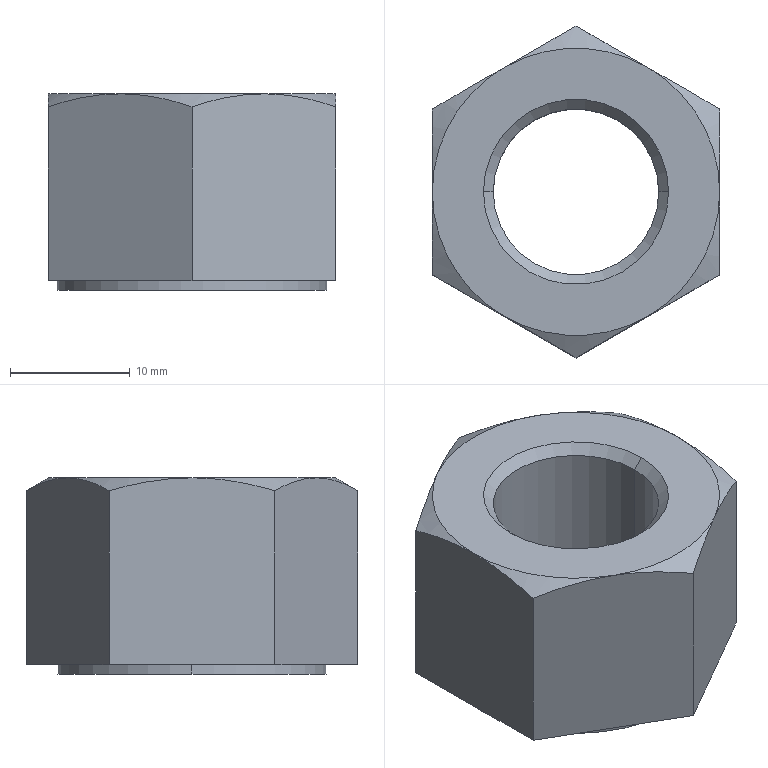Part | SolidWorks | features Cut 2, Chamfer 1, Extrusion 1 | 1 solid | 23 faces | box 24 x 27.713 x 16.4 mm | volume 5589 mm3 | cone 10 | plane 9 | cylinder 4 | commonest cylinder face diameters 13.835 x2 22.5 x2
STEP:
#1=CARTESIAN_POINT('',(-6.918,0.,15.58));
#2=VERTEX_POINT('',#1);
#3=CARTESIAN_POINT('',(6.918,0.,15.58));
#4=VERTEX_POINT('',#3);
#5=CARTESIAN_POINT('',(0.,0.,15.58));
#6=DIRECTION('',(0.,0.,1.));
#7=DIRECTION('',(-1.,0.,0.));
#8=AXIS2_PLACEMENT_3D('',#5,#6,#7);
#9=CIRCLE('',#8,6.918);
#10=EDGE_CURVE('',#2,#4,#9,.T.);
#11=ORIENTED_EDGE('',*,*,#10,.F.);
#12=CARTESIAN_POINT('',(-7.738,0.,16.4));
#13=VERTEX_POINT('',#12);
#14=CARTESIAN_POINT('',(-6.918,0.,15.58));
#15=DIRECTION('',(-0.7071,0.,0.7071));
#16=VECTOR('',#15,1000.);
#17=LINE('',#14,#16);
#18=EDGE_CURVE('',#2,#13,#17,.T.);
#19=ORIENTED_EDGE('',*,*,#18,.T.);
#20=CARTESIAN_POINT('',(7.738,0.,16.4));
#21=VERTEX_POINT('',#20);
#22=CARTESIAN_POINT('',(0.,0.,16.4));
#23=DIRECTION('',(0.,0.,-1.));
#24=DIRECTION('',(-1.,0.,0.));
#25=AXIS2_PLACEMENT_3D('',#22,#23,#24);
#26=CIRCLE('',#25,7.738);
#27=EDGE_CURVE('',#21,#13,#26,.T.);
#28=ORIENTED_EDGE('',*,*,#27,.F.);
#29=CARTESIAN_POINT('',(6.918,0.,15.58));
#30=DIRECTION('',(0.7071,0.,0.7071));
#31=VECTOR('',#30,1000.);
#32=LINE('',#29,#31);
#33=EDGE_CURVE('',#4,#21,#32,.T.);
#34=ORIENTED_EDGE('',*,*,#33,.F.);
#35=EDGE_LOOP('',(#11,#19,#28,#34));
#36=FACE_OUTER_BOUND('',#35,.T.);
#37=CARTESIAN_POINT('',(0.,0.,15.58));
#38=DIRECTION('',(0.,0.,1.));
#39=DIRECTION('',(1.,0.,0.));
#40=AXIS2_PLACEMENT_3D('',#37,#38,#39);
#41=CONICAL_SURFACE('',#40,6.918,0.7854);
#42=ADVANCED_FACE('',(#36),#41,.F.);
#43=CARTESIAN_POINT('',(6.918,0.,0.82));
#44=VERTEX_POINT('',#43);
#45=CARTESIAN_POINT('',(-6.918,0.,0.82));
#46=VERTEX_POINT('',#45);
#47=CARTESIAN_POINT('',(0.,0.,0.82));
#48=DIRECTION('',(0.,0.,-1.));
#49=DIRECTION('',(-1.,0.,0.));
#50=AXIS2_PLACEMENT_3D('',#47,#48,#49);
#51=CIRCLE('',#50,6.918);
#52=EDGE_CURVE('',#44,#46,#51,.T.);
#53=ORIENTED_EDGE('',*,*,#52,.F.);
#54=CARTESIAN_POINT('',(7.738,0.,0.));
#55=VERTEX_POINT('',#54);
#56=CARTESIAN_POINT('',(7.738,0.,0.));
#57=DIRECTION('',(0.7071,0.,-0.7071));
#58=VECTOR('',#57,1000.);
#59=LINE('',#56,#58);
#60=EDGE_CURVE('',#44,#55,#59,.T.);
#61=ORIENTED_EDGE('',*,*,#60,.T.);
#62=CARTESIAN_POINT('',(-7.738,0.,0.));
#63=VERTEX_POINT('',#62);
#64=CARTESIAN_POINT('',(0.,0.,0.));
#65=DIRECTION('',(0.,0.,1.));
#66=DIRECTION('',(-1.,0.,0.));
#67=AXIS2_PLACEMENT_3D('',#64,#65,#66);
#68=CIRCLE('',#67,7.738);
#69=EDGE_CURVE('',#63,#55,#68,.T.);
#70=ORIENTED_EDGE('',*,*,#69,.F.);
#71=CARTESIAN_POINT('',(-7.738,0.,0.));
#72=DIRECTION('',(-0.7071,0.,-0.7071));
#73=VECTOR('',#72,1000.);
#74=LINE('',#71,#73);
#75=EDGE_CURVE('',#46,#63,#74,.T.);
#76=ORIENTED_EDGE('',*,*,#75,.F.);
#77=EDGE_LOOP('',(#53,#61,#70,#76));
#78=FACE_OUTER_BOUND('',#77,.T.);
#79=CARTESIAN_POINT('',(0.,0.,0.));
#80=DIRECTION('',(0.,0.,-1.));
#81=DIRECTION('',(-1.,0.,0.));
#82=AXIS2_PLACEMENT_3D('',#79,#80,#81);
#83=CONICAL_SURFACE('',#82,7.738,0.7854);
#84=ADVANCED_FACE('',(#78),#83,.F.);
#85=CARTESIAN_POINT('',(11.25,0.,0.8));
#86=VERTEX_POINT('',#85);
#87=CARTESIAN_POINT('',(-11.25,0.,0.8));
#88=VERTEX_POINT('',#87);
#89=CARTESIAN_POINT('',(0.,0.,0.8));
#90=DIRECTION('',(0.,0.,1.));
#91=DIRECTION('',(1.,0.,0.));
#92=AXIS2_PLACEMENT_3D('',#89,#90,#91);
#93=CIRCLE('',#92,11.25);
#94=EDGE_CURVE('',#86,#88,#93,.T.);
#95=ORIENTED_EDGE('',*,*,#94,.F.);
#96=CARTESIAN_POINT('',(11.25,0.,0.));
#97=VERTEX_POINT('',#96);
#98=CARTESIAN_POINT('',(11.25,0.,0.8));
#99=DIRECTION('',(0.,0.,-1.));
#100=VECTOR('',#99,1000.);
#101=LINE('',#98,#100);
#102=EDGE_CURVE('',#86,#97,#101,.T.);
#103=ORIENTED_EDGE('',*,*,#102,.T.);
#104=CARTESIAN_POINT('',(-11.25,0.,0.));
#105=VERTEX_POINT('',#104);
#106=CARTESIAN_POINT('',(0.,0.,0.));
#107=DIRECTION('',(0.,0.,1.));
#108=DIRECTION('',(1.,0.,0.));
#109=AXIS2_PLACEMENT_3D('',#106,#107,#108);
#110=CIRCLE('',#109,11.25);
#111=EDGE_CURVE('',#97,#105,#110,.T.);
#112=ORIENTED_EDGE('',*,*,#111,.T.);
#113=CARTESIAN_POINT('',(-11.25,0.,0.8));
#114=DIRECTION('',(0.,0.,-1.));
#115=VECTOR('',#114,1000.);
#116=LINE('',#113,#115);
#117=EDGE_CURVE('',#88,#105,#116,.T.);
#118=ORIENTED_EDGE('',*,*,#117,.F.);
#119=EDGE_LOOP('',(#95,#103,#112,#118));
#120=FACE_OUTER_BOUND('',#119,.T.);
#121=CARTESIAN_POINT('',(0.,0.,0.8));
#122=DIRECTION('',(0.,0.,-1.));
#123=DIRECTION('',(-1.,0.,0.));
#124=AXIS2_PLACEMENT_3D('',#121,#122,#123);
#125=CYLINDRICAL_SURFACE('',#124,11.25);
#126=ADVANCED_FACE('',(#120),#125,.T.);
#127=ORIENTED_EDGE('',*,*,#10,.T.);
#128=CARTESIAN_POINT('',(6.918,0.,16.4));
#129=DIRECTION('',(0.,0.,-1.));
#130=VECTOR('',#129,1000.);
#131=LINE('',#128,#130);
#132=EDGE_CURVE('',#4,#44,#131,.T.);
#133=ORIENTED_EDGE('',*,*,#132,.T.);
#134=ORIENTED_EDGE('',*,*,#52,.T.);
#135=CARTESIAN_POINT('',(-6.918,0.,16.4));
#136=DIRECTION('',(0.,0.,-1.));
#137=VECTOR('',#136,1000.);
#138=LINE('',#135,#137);
#139=EDGE_CURVE('',#2,#46,#138,.T.);
#140=ORIENTED_EDGE('',*,*,#139,.F.);
#141=EDGE_LOOP('',(#127,#133,#134,#140));
#142=FACE_OUTER_BOUND('',#141,.T.);
#143=CARTESIAN_POINT('',(0.,0.,16.4));
#144=DIRECTION('',(0.,0.,-1.));
#145=DIRECTION('',(-1.,0.,0.));
#146=AXIS2_PLACEMENT_3D('',#143,#144,#145);
#147=CYLINDRICAL_SURFACE('',#146,6.918);
#148=ADVANCED_FACE('',(#142),#147,.F.);
#149=ORIENTED_EDGE('',*,*,#27,.T.);
#150=CARTESIAN_POINT('',(0.,0.,16.4));
#151=DIRECTION('',(0.,0.,-1.));
#152=DIRECTION('',(-1.,0.,0.));
#153=AXIS2_PLACEMENT_3D('',#150,#151,#152);
#154=CIRCLE('',#153,7.738);
#155=EDGE_CURVE('',#13,#21,#154,.T.);
#156=ORIENTED_EDGE('',*,*,#155,.T.);
#157=EDGE_LOOP('',(#149,#156));
#158=FACE_BOUND('',#157,.T.);
#159=CARTESIAN_POINT('',(-6.,10.392,16.4));
#160=VERTEX_POINT('',#159);
#161=CARTESIAN_POINT('',(-12.,0.,16.4));
#162=VERTEX_POINT('',#161);
#163=CARTESIAN_POINT('',(0.,0.,16.4));
#164=DIRECTION('',(0.,0.,1.));
#165=DIRECTION('',(1.,0.,0.));
#166=AXIS2_PLACEMENT_3D('',#163,#164,#165);
#167=CIRCLE('',#166,12.);
#168=EDGE_CURVE('',#160,#162,#167,.T.);
#169=ORIENTED_EDGE('',*,*,#168,.T.);
#170=CARTESIAN_POINT('',(-6.,-10.392,16.4));
#171=VERTEX_POINT('',#170);
#172=CARTESIAN_POINT('',(0.,0.,16.4));
#173=DIRECTION('',(0.,0.,1.));
#174=DIRECTION('',(1.,0.,0.));
#175=AXIS2_PLACEMENT_3D('',#172,#173,#174);
#176=CIRCLE('',#175,12.);
#177=EDGE_CURVE('',#162,#171,#176,.T.);
#178=ORIENTED_EDGE('',*,*,#177,.T.);
#179=CARTESIAN_POINT('',(6.,-10.392,16.4));
#180=VERTEX_POINT('',#179);
#181=CARTESIAN_POINT('',(0.,0.,16.4));
#182=DIRECTION('',(0.,0.,1.));
#183=DIRECTION('',(1.,0.,0.));
#184=AXIS2_PLACEMENT_3D('',#181,#182,#183);
#185=CIRCLE('',#184,12.);
#186=EDGE_CURVE('',#171,#180,#185,.T.);
#187=ORIENTED_EDGE('',*,*,#186,.T.);
#188=CARTESIAN_POINT('',(12.,0.,16.4));
#189=VERTEX_POINT('',#188);
#190=CARTESIAN_POINT('',(0.,0.,16.4));
#191=DIRECTION('',(0.,0.,1.));
#192=DIRECTION('',(1.,0.,0.));
#193=AXIS2_PLACEMENT_3D('',#190,#191,#192);
#194=CIRCLE('',#193,12.);
#195=EDGE_CURVE('',#180,#189,#194,.T.);
#196=ORIENTED_EDGE('',*,*,#195,.T.);
#197=CARTESIAN_POINT('',(6.,10.392,16.4));
#198=VERTEX_POINT('',#197);
#199=CARTESIAN_POINT('',(0.,0.,16.4));
#200=DIRECTION('',(0.,0.,1.));
#201=DIRECTION('',(1.,0.,0.));
#202=AXIS2_PLACEMENT_3D('',#199,#200,#201);
#203=CIRCLE('',#202,12.);
#204=EDGE_CURVE('',#189,#198,#203,.T.);
#205=ORIENTED_EDGE('',*,*,#204,.T.);
#206=CARTESIAN_POINT('',(0.,0.,16.4));
#207=DIRECTION('',(0.,0.,1.));
#208=DIRECTION('',(1.,0.,0.));
#209=AXIS2_PLACEMENT_3D('',#206,#207,#208);
#210=CIRCLE('',#209,12.);
#211=EDGE_CURVE('',#198,#160,#210,.T.);
#212=ORIENTED_EDGE('',*,*,#211,.T.);
#213=EDGE_LOOP('',(#169,#178,#187,#196,#205,#212));
#214=FACE_OUTER_BOUND('',#213,.T.);
#215=CARTESIAN_POINT('',(12.,6.928,16.4));
#216=DIRECTION('',(0.,0.,-1.));
#217=DIRECTION('',(-1.,0.,0.));
#218=AXIS2_PLACEMENT_3D('',#215,#216,#217);
#219=PLANE('',#218);
#220=ADVANCED_FACE('',(#158,#214),#219,.F.);
#221=CARTESIAN_POINT('',(12.,6.928,15.328));
#222=VERTEX_POINT('',#221);
#223=CARTESIAN_POINT('',(12.,6.928,15.328));
#224=CARTESIAN_POINT('',(11.018,7.495,15.655));
#225=CARTESIAN_POINT('',(10.03,8.066,15.925));
#226=CARTESIAN_POINT('',(8.032,9.219,16.298));
#227=CARTESIAN_POINT('',(7.022,9.802,16.4));
#228=CARTESIAN_POINT('',(6.,10.392,16.4));
#229=B_SPLINE_CURVE_WITH_KNOTS('',3,(#223,#224,#225,#226,#227,#228),.UNSPECIFIED.,.F.,.F.,(4,2,4),(0.000000238,0.003505,0.00701),.UNSPECIFIED.);
#230=EDGE_CURVE('',#222,#198,#229,.T.);
#231=ORIENTED_EDGE('',*,*,#230,.F.);
#232=CARTESIAN_POINT('',(12.,6.928,0.8));
#233=VERTEX_POINT('',#232);
#234=CARTESIAN_POINT('',(12.,6.928,16.4));
#235=DIRECTION('',(0.,0.,-1.));
#236=VECTOR('',#235,1000.);
#237=LINE('',#234,#236);
#238=EDGE_CURVE('',#222,#233,#237,.T.);
#239=ORIENTED_EDGE('',*,*,#238,.T.);
#240=CARTESIAN_POINT('',(0.,13.856,0.8));
#241=VERTEX_POINT('',#240);
#242=CARTESIAN_POINT('',(12.,6.928,0.8));
#243=DIRECTION('',(-0.866,0.5,0.));
#244=VECTOR('',#243,1000.);
#245=LINE('',#242,#244);
#246=EDGE_CURVE('',#233,#241,#245,.T.);
#247=ORIENTED_EDGE('',*,*,#246,.T.);
#248=CARTESIAN_POINT('',(0.,13.856,15.328));
#249=VERTEX_POINT('',#248);
#250=CARTESIAN_POINT('',(0.,13.856,16.4));
#251=DIRECTION('',(0.,0.,-1.));
#252=VECTOR('',#251,1000.);
#253=LINE('',#250,#252);
#254=EDGE_CURVE('',#249,#241,#253,.T.);
#255=ORIENTED_EDGE('',*,*,#254,.F.);
#256=CARTESIAN_POINT('',(6.,10.392,16.4));
#257=CARTESIAN_POINT('',(5.491,10.686,16.4));
#258=CARTESIAN_POINT('',(4.979,10.982,16.375));
#259=CARTESIAN_POINT('',(3.967,11.566,16.277));
#260=CARTESIAN_POINT('',(3.465,11.856,16.204));
#261=CARTESIAN_POINT('',(1.966,12.721,15.924));
#262=CARTESIAN_POINT('',(0.9791,13.291,15.655));
#263=CARTESIAN_POINT('',(0.,13.856,15.328));
#264=B_SPLINE_CURVE_WITH_KNOTS('',3,(#256,#257,#258,#259,#260,#261,#262,#263),.UNSPECIFIED.,.F.,.F.,(4,2,2,4),(0.00701,0.008756,0.0105,0.01399),.UNSPECIFIED.);
#265=EDGE_CURVE('',#198,#249,#264,.T.);
#266=ORIENTED_EDGE('',*,*,#265,.F.);
#267=EDGE_LOOP('',(#231,#239,#247,#255,#266));
#268=FACE_OUTER_BOUND('',#267,.T.);
#269=CARTESIAN_POINT('',(12.,6.928,16.4));
#270=DIRECTION('',(-0.5,-0.866,0.));
#271=DIRECTION('',(0.866,-0.5,0.));
#272=AXIS2_PLACEMENT_3D('',#269,#270,#271);
#273=PLANE('',#272);
#274=ADVANCED_FACE('',(#268),#273,.F.);
#275=CARTESIAN_POINT('',(0.,13.856,15.328));
#276=CARTESIAN_POINT('',(-0.9815,13.29,15.655));
#277=CARTESIAN_POINT('',(-1.97,12.719,15.925));
#278=CARTESIAN_POINT('',(-3.968,11.565,16.298));
#279=CARTESIAN_POINT('',(-4.978,10.982,16.4));
#280=CARTESIAN_POINT('',(-6.,10.392,16.4));
#281=B_SPLINE_CURVE_WITH_KNOTS('',3,(#275,#276,#277,#278,#279,#280),.UNSPECIFIED.,.F.,.F.,(4,2,4),(0.000000238,0.003505,0.00701),.UNSPECIFIED.);
#282=EDGE_CURVE('',#249,#160,#281,.T.);
#283=ORIENTED_EDGE('',*,*,#282,.F.);
#284=ORIENTED_EDGE('',*,*,#254,.T.);
#285=CARTESIAN_POINT('',(-12.,6.928,0.8));
#286=VERTEX_POINT('',#285);
#287=CARTESIAN_POINT('',(0.,13.856,0.8));
#288=DIRECTION('',(-0.866,-0.5,0.));
#289=VECTOR('',#288,1000.);
#290=LINE('',#287,#289);
#291=EDGE_CURVE('',#241,#286,#290,.T.);
#292=ORIENTED_EDGE('',*,*,#291,.T.);
#293=CARTESIAN_POINT('',(-12.,6.928,15.328));
#294=VERTEX_POINT('',#293);
#295=CARTESIAN_POINT('',(-12.,6.928,16.4));
#296=DIRECTION('',(0.,0.,-1.));
#297=VECTOR('',#296,1000.);
#298=LINE('',#295,#297);
#299=EDGE_CURVE('',#294,#286,#298,.T.);
#300=ORIENTED_EDGE('',*,*,#299,.F.);
#301=CARTESIAN_POINT('',(-6.,10.392,16.4));
#302=CARTESIAN_POINT('',(-6.509,10.098,16.4));
#303=CARTESIAN_POINT('',(-7.021,9.803,16.375));
#304=CARTESIAN_POINT('',(-8.033,9.219,16.277));
#305=CARTESIAN_POINT('',(-8.535,8.929,16.204));
#306=CARTESIAN_POINT('',(-10.034,8.063,15.924));
#307=CARTESIAN_POINT('',(-11.021,7.493,15.655));
#308=CARTESIAN_POINT('',(-12.,6.928,15.328));
#309=B_SPLINE_CURVE_WITH_KNOTS('',3,(#301,#302,#303,#304,#305,#306,#307,#308),.UNSPECIFIED.,.F.,.F.,(4,2,2,4),(0.00701,0.008756,0.0105,0.01399),.UNSPECIFIED.);
#310=EDGE_CURVE('',#160,#294,#309,.T.);
#311=ORIENTED_EDGE('',*,*,#310,.F.);
#312=EDGE_LOOP('',(#283,#284,#292,#300,#311));
#313=FACE_OUTER_BOUND('',#312,.T.);
#314=CARTESIAN_POINT('',(0.,13.856,16.4));
#315=DIRECTION('',(0.5,-0.866,0.));
#316=DIRECTION('',(0.866,0.5,0.));
#317=AXIS2_PLACEMENT_3D('',#314,#315,#316);
#318=PLANE('',#317);
#319=ADVANCED_FACE('',(#313),#318,.F.);
#320=CARTESIAN_POINT('',(-12.,6.928,15.328));
#321=CARTESIAN_POINT('',(-12.,5.808,15.652));
#322=CARTESIAN_POINT('',(-12.,4.673,15.921));
#323=CARTESIAN_POINT('',(-12.,2.939,16.202));
#324=CARTESIAN_POINT('',(-12.,2.355,16.276));
#325=CARTESIAN_POINT('',(-12.,1.176,16.375));
#326=CARTESIAN_POINT('',(-12.,0.5864,16.4));
#327=CARTESIAN_POINT('',(-12.,0.,16.4));
#328=B_SPLINE_CURVE_WITH_KNOTS('',3,(#320,#321,#322,#323,#324,#325,#326,#327),.UNSPECIFIED.,.F.,.F.,(4,2,2,4),(0.04083,0.04433,0.04609,0.04784),.UNSPECIFIED.);
#329=EDGE_CURVE('',#294,#162,#328,.T.);
#330=ORIENTED_EDGE('',*,*,#329,.F.);
#331=ORIENTED_EDGE('',*,*,#299,.T.);
#332=CARTESIAN_POINT('',(-12.,-6.928,0.8));
#333=VERTEX_POINT('',#332);
#334=CARTESIAN_POINT('',(-12.,6.928,0.8));
#335=DIRECTION('',(0.,-1.,0.));
#336=VECTOR('',#335,1000.);
#337=LINE('',#334,#336);
#338=EDGE_CURVE('',#286,#333,#337,.T.);
#339=ORIENTED_EDGE('',*,*,#338,.T.);
#340=CARTESIAN_POINT('',(-12.,-6.928,15.328));
#341=VERTEX_POINT('',#340);
#342=CARTESIAN_POINT('',(-12.,-6.928,16.4));
#343=DIRECTION('',(0.,0.,-1.));
#344=VECTOR('',#343,1000.);
#345=LINE('',#342,#344);
#346=EDGE_CURVE('',#341,#333,#345,.T.);
#347=ORIENTED_EDGE('',*,*,#346,.F.);
#348=CARTESIAN_POINT('',(-12.,0.,16.4));
#349=CARTESIAN_POINT('',(-12.,-1.172,16.4));
#350=CARTESIAN_POINT('',(-12.,-2.335,16.299));
#351=CARTESIAN_POINT('',(-12.,-4.647,15.926));
#352=CARTESIAN_POINT('',(-12.,-5.8,15.654));
#353=CARTESIAN_POINT('',(-12.,-6.928,15.328));
#354=B_SPLINE_CURVE_WITH_KNOTS('',3,(#348,#349,#350,#351,#352,#353),.UNSPECIFIED.,.F.,.F.,(4,2,4),(0.04784,0.05135,0.05485),.UNSPECIFIED.);
#355=EDGE_CURVE('',#162,#341,#354,.T.);
#356=ORIENTED_EDGE('',*,*,#355,.F.);
#357=EDGE_LOOP('',(#330,#331,#339,#347,#356));
#358=FACE_OUTER_BOUND('',#357,.T.);
#359=CARTESIAN_POINT('',(-12.,6.928,16.4));
#360=DIRECTION('',(1.,0.,0.));
#361=DIRECTION('',(0.,0.,-1.));
#362=AXIS2_PLACEMENT_3D('',#359,#360,#361);
#363=PLANE('',#362);
#364=ADVANCED_FACE('',(#358),#363,.F.);
#365=CARTESIAN_POINT('',(-12.,-6.928,15.328));
#366=CARTESIAN_POINT('',(-11.018,-7.495,15.655));
#367=CARTESIAN_POINT('',(-10.03,-8.066,15.925));
#368=CARTESIAN_POINT('',(-8.032,-9.219,16.298));
#369=CARTESIAN_POINT('',(-7.022,-9.802,16.4));
#370=CARTESIAN_POINT('',(-6.,-10.392,16.4));
#371=B_SPLINE_CURVE_WITH_KNOTS('',3,(#365,#366,#367,#368,#369,#370),.UNSPECIFIED.,.F.,.F.,(4,2,4),(0.000000238,0.003505,0.00701),.UNSPECIFIED.);
#372=EDGE_CURVE('',#341,#171,#371,.T.);
#373=ORIENTED_EDGE('',*,*,#372,.F.);
#374=ORIENTED_EDGE('',*,*,#346,.T.);
#375=CARTESIAN_POINT('',(0.,-13.856,0.8));
#376=VERTEX_POINT('',#375);
#377=CARTESIAN_POINT('',(-12.,-6.928,0.8));
#378=DIRECTION('',(0.866,-0.5,0.));
#379=VECTOR('',#378,1000.);
#380=LINE('',#377,#379);
#381=EDGE_CURVE('',#333,#376,#380,.T.);
#382=ORIENTED_EDGE('',*,*,#381,.T.);
#383=CARTESIAN_POINT('',(0.,-13.856,15.328));
#384=VERTEX_POINT('',#383);
#385=CARTESIAN_POINT('',(0.,-13.856,16.4));
#386=DIRECTION('',(0.,0.,-1.));
#387=VECTOR('',#386,1000.);
#388=LINE('',#385,#387);
#389=EDGE_CURVE('',#384,#376,#388,.T.);
#390=ORIENTED_EDGE('',*,*,#389,.F.);
#391=CARTESIAN_POINT('',(-6.,-10.392,16.4));
#392=CARTESIAN_POINT('',(-5.491,-10.686,16.4));
#393=CARTESIAN_POINT('',(-4.979,-10.982,16.375));
#394=CARTESIAN_POINT('',(-3.967,-11.566,16.277));
#395=CARTESIAN_POINT('',(-3.465,-11.856,16.204));
#396=CARTESIAN_POINT('',(-1.966,-12.721,15.924));
#397=CARTESIAN_POINT('',(-0.9791,-13.291,15.655));
#398=CARTESIAN_POINT('',(0.,-13.856,15.328));
#399=B_SPLINE_CURVE_WITH_KNOTS('',3,(#391,#392,#393,#394,#395,#396,#397,#398),.UNSPECIFIED.,.F.,.F.,(4,2,2,4),(0.00701,0.008756,0.0105,0.01399),.UNSPECIFIED.);
#400=EDGE_CURVE('',#171,#384,#399,.T.);
#401=ORIENTED_EDGE('',*,*,#400,.F.);
#402=EDGE_LOOP('',(#373,#374,#382,#390,#401));
#403=FACE_OUTER_BOUND('',#402,.T.);
#404=CARTESIAN_POINT('',(-12.,-6.928,16.4));
#405=DIRECTION('',(0.5,0.866,0.));
#406=DIRECTION('',(-0.866,0.5,0.));
#407=AXIS2_PLACEMENT_3D('',#404,#405,#406);
#408=PLANE('',#407);
#409=ADVANCED_FACE('',(#403),#408,.F.);
#410=CARTESIAN_POINT('',(0.,-13.856,15.328));
#411=CARTESIAN_POINT('',(0.9815,-13.29,15.655));
#412=CARTESIAN_POINT('',(1.97,-12.719,15.925));
#413=CARTESIAN_POINT('',(3.968,-11.565,16.298));
#414=CARTESIAN_POINT('',(4.978,-10.982,16.4));
#415=CARTESIAN_POINT('',(6.,-10.392,16.4));
#416=B_SPLINE_CURVE_WITH_KNOTS('',3,(#410,#411,#412,#413,#414,#415),.UNSPECIFIED.,.F.,.F.,(4,2,4),(0.000000238,0.003505,0.00701),.UNSPECIFIED.);
#417=EDGE_CURVE('',#384,#180,#416,.T.);
#418=ORIENTED_EDGE('',*,*,#417,.F.);
#419=ORIENTED_EDGE('',*,*,#389,.T.);
#420=CARTESIAN_POINT('',(12.,-6.928,0.8));
#421=VERTEX_POINT('',#420);
#422=CARTESIAN_POINT('',(0.,-13.856,0.8));
#423=DIRECTION('',(0.866,0.5,0.));
#424=VECTOR('',#423,1000.);
#425=LINE('',#422,#424);
#426=EDGE_CURVE('',#376,#421,#425,.T.);
#427=ORIENTED_EDGE('',*,*,#426,.T.);
#428=CARTESIAN_POINT('',(12.,-6.928,15.328));
#429=VERTEX_POINT('',#428);
#430=CARTESIAN_POINT('',(12.,-6.928,16.4));
#431=DIRECTION('',(0.,0.,-1.));
#432=VECTOR('',#431,1000.);
#433=LINE('',#430,#432);
#434=EDGE_CURVE('',#429,#421,#433,.T.);
#435=ORIENTED_EDGE('',*,*,#434,.F.);
#436=CARTESIAN_POINT('',(6.,-10.392,16.4));
#437=CARTESIAN_POINT('',(6.509,-10.098,16.4));
#438=CARTESIAN_POINT('',(7.021,-9.803,16.375));
#439=CARTESIAN_POINT('',(8.033,-9.219,16.277));
#440=CARTESIAN_POINT('',(8.535,-8.929,16.204));
#441=CARTESIAN_POINT('',(10.034,-8.063,15.924));
#442=CARTESIAN_POINT('',(11.021,-7.493,15.655));
#443=CARTESIAN_POINT('',(12.,-6.928,15.328));
#444=B_SPLINE_CURVE_WITH_KNOTS('',3,(#436,#437,#438,#439,#440,#441,#442,#443),.UNSPECIFIED.,.F.,.F.,(4,2,2,4),(0.00701,0.008756,0.0105,0.01399),.UNSPECIFIED.);
#445=EDGE_CURVE('',#180,#429,#444,.T.);
#446=ORIENTED_EDGE('',*,*,#445,.F.);
#447=EDGE_LOOP('',(#418,#419,#427,#435,#446));
#448=FACE_OUTER_BOUND('',#447,.T.);
#449=CARTESIAN_POINT('',(0.,-13.856,16.4));
#450=DIRECTION('',(-0.5,0.866,0.));
#451=DIRECTION('',(-0.866,-0.5,0.));
#452=AXIS2_PLACEMENT_3D('',#449,#450,#451);
#453=PLANE('',#452);
#454=ADVANCED_FACE('',(#448),#453,.F.);
#455=CARTESIAN_POINT('',(12.,-6.928,15.328));
#456=CARTESIAN_POINT('',(12.,-5.8,15.654));
#457=CARTESIAN_POINT('',(12.,-4.647,15.926));
#458=CARTESIAN_POINT('',(12.,-2.335,16.299));
#459=CARTESIAN_POINT('',(12.,-1.172,16.4));
#460=CARTESIAN_POINT('',(12.,0.,16.4));
#461=B_SPLINE_CURVE_WITH_KNOTS('',3,(#455,#456,#457,#458,#459,#460),.UNSPECIFIED.,.F.,.F.,(4,2,4),(0.01275,0.01625,0.01976),.UNSPECIFIED.);
#462=EDGE_CURVE('',#429,#189,#461,.T.);
#463=ORIENTED_EDGE('',*,*,#462,.F.);
#464=ORIENTED_EDGE('',*,*,#434,.T.);
#465=CARTESIAN_POINT('',(12.,-6.928,0.8));
#466=DIRECTION('',(0.,1.,0.));
#467=VECTOR('',#466,1000.);
#468=LINE('',#465,#467);
#469=EDGE_CURVE('',#421,#233,#468,.T.);
#470=ORIENTED_EDGE('',*,*,#469,.T.);
#471=ORIENTED_EDGE('',*,*,#238,.F.);
#472=CARTESIAN_POINT('',(12.,0.,16.4));
#473=CARTESIAN_POINT('',(12.,0.5864,16.4));
#474=CARTESIAN_POINT('',(12.,1.176,16.375));
#475=CARTESIAN_POINT('',(12.,2.355,16.276));
#476=CARTESIAN_POINT('',(12.,2.939,16.202));
#477=CARTESIAN_POINT('',(12.,4.673,15.921));
#478=CARTESIAN_POINT('',(12.,5.808,15.652));
#479=CARTESIAN_POINT('',(12.,6.928,15.328));
#480=B_SPLINE_CURVE_WITH_KNOTS('',3,(#472,#473,#474,#475,#476,#477,#478,#479),.UNSPECIFIED.,.F.,.F.,(4,2,2,4),(0.01976,0.02151,0.02327,0.02678),.UNSPECIFIED.);
#481=EDGE_CURVE('',#189,#222,#480,.T.);
#482=ORIENTED_EDGE('',*,*,#481,.F.);
#483=EDGE_LOOP('',(#463,#464,#470,#471,#482));
#484=FACE_OUTER_BOUND('',#483,.T.);
#485=CARTESIAN_POINT('',(12.,-6.928,16.4));
#486=DIRECTION('',(-1.,0.,0.));
#487=DIRECTION('',(0.,-1.,0.));
#488=AXIS2_PLACEMENT_3D('',#485,#486,#487);
#489=PLANE('',#488);
#490=ADVANCED_FACE('',(#484),#489,.F.);
#491=ORIENTED_EDGE('',*,*,#69,.T.);
#492=CARTESIAN_POINT('',(0.,0.,0.));
#493=DIRECTION('',(0.,0.,1.));
#494=DIRECTION('',(-1.,0.,0.));
#495=AXIS2_PLACEMENT_3D('',#492,#493,#494);
#496=CIRCLE('',#495,7.738);
#497=EDGE_CURVE('',#55,#63,#496,.T.);
#498=ORIENTED_EDGE('',*,*,#497,.T.);
#499=EDGE_LOOP('',(#491,#498));
#500=FACE_BOUND('',#499,.T.);
#501=CARTESIAN_POINT('',(0.,0.,0.));
#502=DIRECTION('',(0.,0.,1.));
#503=DIRECTION('',(1.,0.,0.));
#504=AXIS2_PLACEMENT_3D('',#501,#502,#503);
#505=CIRCLE('',#504,11.25);
#506=EDGE_CURVE('',#105,#97,#505,.T.);
#507=ORIENTED_EDGE('',*,*,#506,.F.);
#508=ORIENTED_EDGE('',*,*,#111,.F.);
#509=EDGE_LOOP('',(#507,#508));
#510=FACE_OUTER_BOUND('',#509,.T.);
#511=CARTESIAN_POINT('',(12.,6.928,0.));
#512=DIRECTION('',(0.,0.,-1.));
#513=DIRECTION('',(-1.,0.,0.));
#514=AXIS2_PLACEMENT_3D('',#511,#512,#513);
#515=PLANE('',#514);
#516=ADVANCED_FACE('',(#500,#510),#515,.T.);
#517=ORIENTED_EDGE('',*,*,#132,.F.);
#518=CARTESIAN_POINT('',(0.,0.,15.58));
#519=DIRECTION('',(0.,0.,1.));
#520=DIRECTION('',(-1.,0.,0.));
#521=AXIS2_PLACEMENT_3D('',#518,#519,#520);
#522=CIRCLE('',#521,6.918);
#523=EDGE_CURVE('',#4,#2,#522,.T.);
#524=ORIENTED_EDGE('',*,*,#523,.T.);
#525=ORIENTED_EDGE('',*,*,#139,.T.);
#526=CARTESIAN_POINT('',(0.,0.,0.82));
#527=DIRECTION('',(0.,0.,-1.));
#528=DIRECTION('',(-1.,0.,0.));
#529=AXIS2_PLACEMENT_3D('',#526,#527,#528);
#530=CIRCLE('',#529,6.918);
#531=EDGE_CURVE('',#46,#44,#530,.T.);
#532=ORIENTED_EDGE('',*,*,#531,.T.);
#533=EDGE_LOOP('',(#517,#524,#525,#532));
#534=FACE_OUTER_BOUND('',#533,.T.);
#535=CARTESIAN_POINT('',(0.,0.,16.4));
#536=DIRECTION('',(0.,0.,-1.));
#537=DIRECTION('',(-1.,0.,0.));
#538=AXIS2_PLACEMENT_3D('',#535,#536,#537);
#539=CYLINDRICAL_SURFACE('',#538,6.918);
#540=ADVANCED_FACE('',(#534),#539,.F.);
#541=CARTESIAN_POINT('',(0.,0.,0.8));
#542=DIRECTION('',(0.,0.,1.));
#543=DIRECTION('',(1.,0.,0.));
#544=AXIS2_PLACEMENT_3D('',#541,#542,#543);
#545=CIRCLE('',#544,11.25);
#546=EDGE_CURVE('',#88,#86,#545,.T.);
#547=ORIENTED_EDGE('',*,*,#546,.T.);
#548=ORIENTED_EDGE('',*,*,#94,.T.);
#549=EDGE_LOOP('',(#547,#548));
#550=FACE_BOUND('',#549,.T.);
#551=ORIENTED_EDGE('',*,*,#469,.F.);
#552=ORIENTED_EDGE('',*,*,#426,.F.);
#553=ORIENTED_EDGE('',*,*,#381,.F.);
#554=ORIENTED_EDGE('',*,*,#338,.F.);
#555=ORIENTED_EDGE('',*,*,#291,.F.);
#556=ORIENTED_EDGE('',*,*,#246,.F.);
#557=EDGE_LOOP('',(#551,#552,#553,#554,#555,#556));
#558=FACE_OUTER_BOUND('',#557,.T.);
#559=CARTESIAN_POINT('',(0.,0.,0.8));
#560=DIRECTION('',(0.,0.,1.));
#561=DIRECTION('',(1.,0.,0.));
#562=AXIS2_PLACEMENT_3D('',#559,#560,#561);
#563=PLANE('',#562);
#564=ADVANCED_FACE('',(#550,#558),#563,.F.);
#565=ORIENTED_EDGE('',*,*,#102,.F.);
#566=ORIENTED_EDGE('',*,*,#546,.F.);
#567=ORIENTED_EDGE('',*,*,#117,.T.);
#568=ORIENTED_EDGE('',*,*,#506,.T.);
#569=EDGE_LOOP('',(#565,#566,#567,#568));
#570=FACE_OUTER_BOUND('',#569,.T.);
#571=CARTESIAN_POINT('',(0.,0.,0.8));
#572=DIRECTION('',(0.,0.,-1.));
#573=DIRECTION('',(-1.,0.,0.));
#574=AXIS2_PLACEMENT_3D('',#571,#572,#573);
#575=CYLINDRICAL_SURFACE('',#574,11.25);
#576=ADVANCED_FACE('',(#570),#575,.T.);
#577=ORIENTED_EDGE('',*,*,#230,.T.);
#578=ORIENTED_EDGE('',*,*,#204,.F.);
#579=ORIENTED_EDGE('',*,*,#481,.T.);
#580=EDGE_LOOP('',(#577,#578,#579));
#581=FACE_OUTER_BOUND('',#580,.T.);
#582=CARTESIAN_POINT('',(0.,0.,16.4));
#583=DIRECTION('',(0.,0.,-1.));
#584=DIRECTION('',(1.,0.,0.));
#585=AXIS2_PLACEMENT_3D('',#582,#583,#584);
#586=CONICAL_SURFACE('',#585,12.,1.047);
#587=ADVANCED_FACE('',(#581),#586,.T.);
#588=ORIENTED_EDGE('',*,*,#445,.T.);
#589=ORIENTED_EDGE('',*,*,#462,.T.);
#590=ORIENTED_EDGE('',*,*,#195,.F.);
#591=EDGE_LOOP('',(#588,#589,#590));
#592=FACE_OUTER_BOUND('',#591,.T.);
#593=CARTESIAN_POINT('',(0.,0.,16.4));
#594=DIRECTION('',(0.,0.,-1.));
#595=DIRECTION('',(1.,0.,0.));
#596=AXIS2_PLACEMENT_3D('',#593,#594,#595);
#597=CONICAL_SURFACE('',#596,12.,1.047);
#598=ADVANCED_FACE('',(#592),#597,.T.);
#599=ORIENTED_EDGE('',*,*,#400,.T.);
#600=ORIENTED_EDGE('',*,*,#417,.T.);
#601=ORIENTED_EDGE('',*,*,#186,.F.);
#602=EDGE_LOOP('',(#599,#600,#601));
#603=FACE_OUTER_BOUND('',#602,.T.);
#604=CARTESIAN_POINT('',(0.,0.,16.4));
#605=DIRECTION('',(0.,0.,-1.));
#606=DIRECTION('',(1.,0.,0.));
#607=AXIS2_PLACEMENT_3D('',#604,#605,#606);
#608=CONICAL_SURFACE('',#607,12.,1.047);
#609=ADVANCED_FACE('',(#603),#608,.T.);
#610=ORIENTED_EDGE('',*,*,#355,.T.);
#611=ORIENTED_EDGE('',*,*,#372,.T.);
#612=ORIENTED_EDGE('',*,*,#177,.F.);
#613=EDGE_LOOP('',(#610,#611,#612));
#614=FACE_OUTER_BOUND('',#613,.T.);
#615=CARTESIAN_POINT('',(0.,0.,16.4));
#616=DIRECTION('',(0.,0.,-1.));
#617=DIRECTION('',(1.,0.,0.));
#618=AXIS2_PLACEMENT_3D('',#615,#616,#617);
#619=CONICAL_SURFACE('',#618,12.,1.047);
#620=ADVANCED_FACE('',(#614),#619,.T.);
#621=ORIENTED_EDGE('',*,*,#310,.T.);
#622=ORIENTED_EDGE('',*,*,#329,.T.);
#623=ORIENTED_EDGE('',*,*,#168,.F.);
#624=EDGE_LOOP('',(#621,#622,#623));
#625=FACE_OUTER_BOUND('',#624,.T.);
#626=CARTESIAN_POINT('',(0.,0.,16.4));
#627=DIRECTION('',(0.,0.,-1.));
#628=DIRECTION('',(1.,0.,0.));
#629=AXIS2_PLACEMENT_3D('',#626,#627,#628);
#630=CONICAL_SURFACE('',#629,12.,1.047);
#631=ADVANCED_FACE('',(#625),#630,.T.);
#632=ORIENTED_EDGE('',*,*,#265,.T.);
#633=ORIENTED_EDGE('',*,*,#282,.T.);
#634=ORIENTED_EDGE('',*,*,#211,.F.);
#635=EDGE_LOOP('',(#632,#633,#634));
#636=FACE_OUTER_BOUND('',#635,.T.);
#637=CARTESIAN_POINT('',(0.,0.,16.4));
#638=DIRECTION('',(0.,0.,-1.));
#639=DIRECTION('',(1.,0.,0.));
#640=AXIS2_PLACEMENT_3D('',#637,#638,#639);
#641=CONICAL_SURFACE('',#640,12.,1.047);
#642=ADVANCED_FACE('',(#636),#641,.T.);
#643=ORIENTED_EDGE('',*,*,#60,.F.);
#644=ORIENTED_EDGE('',*,*,#531,.F.);
#645=ORIENTED_EDGE('',*,*,#75,.T.);
#646=ORIENTED_EDGE('',*,*,#497,.F.);
#647=EDGE_LOOP('',(#643,#644,#645,#646));
#648=FACE_OUTER_BOUND('',#647,.T.);
#649=CARTESIAN_POINT('',(0.,0.,0.));
#650=DIRECTION('',(0.,0.,-1.));
#651=DIRECTION('',(-1.,0.,0.));
#652=AXIS2_PLACEMENT_3D('',#649,#650,#651);
#653=CONICAL_SURFACE('',#652,7.738,0.7854);
#654=ADVANCED_FACE('',(#648),#653,.F.);
#655=ORIENTED_EDGE('',*,*,#18,.F.);
#656=ORIENTED_EDGE('',*,*,#523,.F.);
#657=ORIENTED_EDGE('',*,*,#33,.T.);
#658=ORIENTED_EDGE('',*,*,#155,.F.);
#659=EDGE_LOOP('',(#655,#656,#657,#658));
#660=FACE_OUTER_BOUND('',#659,.T.);
#661=CARTESIAN_POINT('',(0.,0.,15.58));
#662=DIRECTION('',(0.,0.,1.));
#663=DIRECTION('',(1.,0.,0.));
#664=AXIS2_PLACEMENT_3D('',#661,#662,#663);
#665=CONICAL_SURFACE('',#664,6.918,0.7854);
#666=ADVANCED_FACE('',(#660),#665,.F.);
#667=CLOSED_SHELL('',(#42,#84,#126,#148,#220,#274,#319,#364,#409,#454,#490,#516,#540,#564,#576,#587,#598,#609,#620,#631,#642,#654,#666));
#668=MANIFOLD_SOLID_BREP('',#667);
#669=CARTESIAN_POINT('',(0.,0.,0.));
#670=DIRECTION('',(0.,0.,1.));
#671=DIRECTION('',(1.,0.,0.));
#672=AXIS2_PLACEMENT_3D('',#669,#670,#671);
#673=(LENGTH_UNIT()NAMED_UNIT(*)SI_UNIT(.MILLI.,.METRE.));
#674=UNCERTAINTY_MEASURE_WITH_UNIT(LENGTH_MEASURE(0.00001),#673,'','');
#675=(NAMED_UNIT(*)PLANE_ANGLE_UNIT()SI_UNIT($,.RADIAN.));
#676=(NAMED_UNIT(*)SI_UNIT($,.STERADIAN.)SOLID_ANGLE_UNIT());
#677=(GEOMETRIC_REPRESENTATION_CONTEXT(3)GLOBAL_UNCERTAINTY_ASSIGNED_CONTEXT((#674))GLOBAL_UNIT_ASSIGNED_CONTEXT((#673,#675,#676))REPRESENTATION_CONTEXT('',''));
#678=ADVANCED_BREP_SHAPE_REPRESENTATION('',(#668,#672),#677);